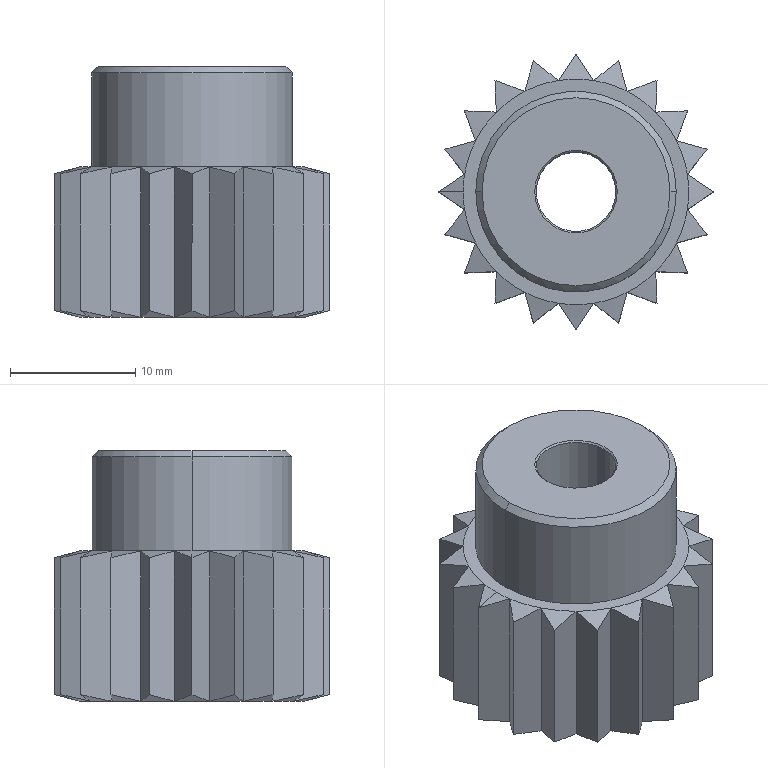Part | STEP file | QA-GER1.0-20-W12-B-H6.35 | 1 solid | 95 faces | box 22 x 22 x 20 mm | volume 4666 mm3 | cone 48 | plane 43 | cylinder 4 | commonest cylinder face diameters 6.35 x2 16 x2